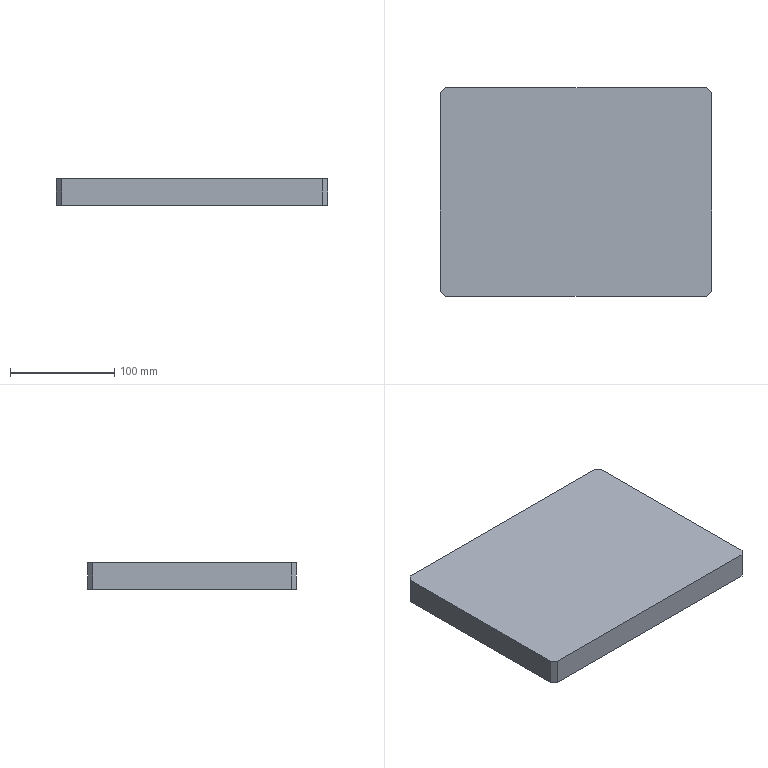Part | SolidWorks | features Chamfer 1, Extrusion 1 | 1 solid | 10 faces | box 260 x 200 x 25 mm | volume 1298750 mm3 | plane 10
STEP:
#1=CARTESIAN_POINT('',(130.,-95.,25.));
#2=VERTEX_POINT('',#1);
#3=CARTESIAN_POINT('',(130.,95.,25.));
#4=VERTEX_POINT('',#3);
#5=CARTESIAN_POINT('',(130.,100.,25.));
#6=DIRECTION('',(0.,1.,0.));
#7=VECTOR('',#6,1000.);
#8=LINE('',#5,#7);
#9=EDGE_CURVE('',#2,#4,#8,.T.);
#10=ORIENTED_EDGE('',*,*,#9,.F.);
#11=CARTESIAN_POINT('',(130.,-95.,0.));
#12=VERTEX_POINT('',#11);
#13=CARTESIAN_POINT('',(130.,-95.,25.));
#14=DIRECTION('',(0.,0.,-1.));
#15=VECTOR('',#14,1000.);
#16=LINE('',#13,#15);
#17=EDGE_CURVE('',#2,#12,#16,.T.);
#18=ORIENTED_EDGE('',*,*,#17,.T.);
#19=CARTESIAN_POINT('',(130.,95.,0.));
#20=VERTEX_POINT('',#19);
#21=CARTESIAN_POINT('',(130.,100.,0.));
#22=DIRECTION('',(0.,1.,0.));
#23=VECTOR('',#22,1000.);
#24=LINE('',#21,#23);
#25=EDGE_CURVE('',#12,#20,#24,.T.);
#26=ORIENTED_EDGE('',*,*,#25,.T.);
#27=CARTESIAN_POINT('',(130.,95.,25.));
#28=DIRECTION('',(0.,0.,1.));
#29=VECTOR('',#28,1000.);
#30=LINE('',#27,#29);
#31=EDGE_CURVE('',#20,#4,#30,.T.);
#32=ORIENTED_EDGE('',*,*,#31,.T.);
#33=EDGE_LOOP('',(#10,#18,#26,#32));
#34=FACE_OUTER_BOUND('',#33,.T.);
#35=CARTESIAN_POINT('',(130.,100.,25.));
#36=DIRECTION('',(-1.,0.,0.));
#37=DIRECTION('',(0.,-1.,0.));
#38=AXIS2_PLACEMENT_3D('',#35,#36,#37);
#39=PLANE('',#38);
#40=ADVANCED_FACE('',(#34),#39,.F.);
#41=CARTESIAN_POINT('',(125.,100.,0.));
#42=VERTEX_POINT('',#41);
#43=CARTESIAN_POINT('',(-125.,100.,0.));
#44=VERTEX_POINT('',#43);
#45=CARTESIAN_POINT('',(-130.,100.,0.));
#46=DIRECTION('',(-1.,0.,0.));
#47=VECTOR('',#46,1000.);
#48=LINE('',#45,#47);
#49=EDGE_CURVE('',#42,#44,#48,.T.);
#50=ORIENTED_EDGE('',*,*,#49,.T.);
#51=CARTESIAN_POINT('',(-125.,100.,25.));
#52=VERTEX_POINT('',#51);
#53=CARTESIAN_POINT('',(-125.,100.,25.));
#54=DIRECTION('',(0.,0.,1.));
#55=VECTOR('',#54,1000.);
#56=LINE('',#53,#55);
#57=EDGE_CURVE('',#44,#52,#56,.T.);
#58=ORIENTED_EDGE('',*,*,#57,.T.);
#59=CARTESIAN_POINT('',(125.,100.,25.));
#60=VERTEX_POINT('',#59);
#61=CARTESIAN_POINT('',(-130.,100.,25.));
#62=DIRECTION('',(-1.,0.,0.));
#63=VECTOR('',#62,1000.);
#64=LINE('',#61,#63);
#65=EDGE_CURVE('',#60,#52,#64,.T.);
#66=ORIENTED_EDGE('',*,*,#65,.F.);
#67=CARTESIAN_POINT('',(125.,100.,25.));
#68=DIRECTION('',(0.,0.,-1.));
#69=VECTOR('',#68,1000.);
#70=LINE('',#67,#69);
#71=EDGE_CURVE('',#60,#42,#70,.T.);
#72=ORIENTED_EDGE('',*,*,#71,.T.);
#73=EDGE_LOOP('',(#50,#58,#66,#72));
#74=FACE_OUTER_BOUND('',#73,.T.);
#75=CARTESIAN_POINT('',(-130.,100.,25.));
#76=DIRECTION('',(0.,-1.,0.));
#77=DIRECTION('',(0.,0.,-1.));
#78=AXIS2_PLACEMENT_3D('',#75,#76,#77);
#79=PLANE('',#78);
#80=ADVANCED_FACE('',(#74),#79,.F.);
#81=CARTESIAN_POINT('',(-130.,95.,0.));
#82=VERTEX_POINT('',#81);
#83=CARTESIAN_POINT('',(-130.,-95.,0.));
#84=VERTEX_POINT('',#83);
#85=CARTESIAN_POINT('',(-130.,100.,0.));
#86=DIRECTION('',(0.,-1.,0.));
#87=VECTOR('',#86,1000.);
#88=LINE('',#85,#87);
#89=EDGE_CURVE('',#82,#84,#88,.T.);
#90=ORIENTED_EDGE('',*,*,#89,.T.);
#91=CARTESIAN_POINT('',(-130.,-95.,25.));
#92=VERTEX_POINT('',#91);
#93=CARTESIAN_POINT('',(-130.,-95.,25.));
#94=DIRECTION('',(0.,0.,1.));
#95=VECTOR('',#94,1000.);
#96=LINE('',#93,#95);
#97=EDGE_CURVE('',#84,#92,#96,.T.);
#98=ORIENTED_EDGE('',*,*,#97,.T.);
#99=CARTESIAN_POINT('',(-130.,95.,25.));
#100=VERTEX_POINT('',#99);
#101=CARTESIAN_POINT('',(-130.,100.,25.));
#102=DIRECTION('',(0.,-1.,0.));
#103=VECTOR('',#102,1000.);
#104=LINE('',#101,#103);
#105=EDGE_CURVE('',#100,#92,#104,.T.);
#106=ORIENTED_EDGE('',*,*,#105,.F.);
#107=CARTESIAN_POINT('',(-130.,95.,25.));
#108=DIRECTION('',(0.,0.,-1.));
#109=VECTOR('',#108,1000.);
#110=LINE('',#107,#109);
#111=EDGE_CURVE('',#100,#82,#110,.T.);
#112=ORIENTED_EDGE('',*,*,#111,.T.);
#113=EDGE_LOOP('',(#90,#98,#106,#112));
#114=FACE_OUTER_BOUND('',#113,.T.);
#115=CARTESIAN_POINT('',(-130.,100.,25.));
#116=DIRECTION('',(1.,0.,0.));
#117=DIRECTION('',(0.,1.,0.));
#118=AXIS2_PLACEMENT_3D('',#115,#116,#117);
#119=PLANE('',#118);
#120=ADVANCED_FACE('',(#114),#119,.F.);
#121=CARTESIAN_POINT('',(-125.,-100.,25.));
#122=VERTEX_POINT('',#121);
#123=CARTESIAN_POINT('',(125.,-100.,25.));
#124=VERTEX_POINT('',#123);
#125=CARTESIAN_POINT('',(-130.,-100.,25.));
#126=DIRECTION('',(1.,0.,0.));
#127=VECTOR('',#126,1000.);
#128=LINE('',#125,#127);
#129=EDGE_CURVE('',#122,#124,#128,.T.);
#130=ORIENTED_EDGE('',*,*,#129,.F.);
#131=CARTESIAN_POINT('',(-125.,-100.,0.));
#132=VERTEX_POINT('',#131);
#133=CARTESIAN_POINT('',(-125.,-100.,25.));
#134=DIRECTION('',(0.,0.,-1.));
#135=VECTOR('',#134,1000.);
#136=LINE('',#133,#135);
#137=EDGE_CURVE('',#122,#132,#136,.T.);
#138=ORIENTED_EDGE('',*,*,#137,.T.);
#139=CARTESIAN_POINT('',(125.,-100.,0.));
#140=VERTEX_POINT('',#139);
#141=CARTESIAN_POINT('',(-130.,-100.,0.));
#142=DIRECTION('',(1.,0.,0.));
#143=VECTOR('',#142,1000.);
#144=LINE('',#141,#143);
#145=EDGE_CURVE('',#132,#140,#144,.T.);
#146=ORIENTED_EDGE('',*,*,#145,.T.);
#147=CARTESIAN_POINT('',(125.,-100.,25.));
#148=DIRECTION('',(0.,0.,1.));
#149=VECTOR('',#148,1000.);
#150=LINE('',#147,#149);
#151=EDGE_CURVE('',#140,#124,#150,.T.);
#152=ORIENTED_EDGE('',*,*,#151,.T.);
#153=EDGE_LOOP('',(#130,#138,#146,#152));
#154=FACE_OUTER_BOUND('',#153,.T.);
#155=CARTESIAN_POINT('',(-130.,-100.,25.));
#156=DIRECTION('',(0.,1.,0.));
#157=DIRECTION('',(0.,0.,1.));
#158=AXIS2_PLACEMENT_3D('',#155,#156,#157);
#159=PLANE('',#158);
#160=ADVANCED_FACE('',(#154),#159,.F.);
#161=ORIENTED_EDGE('',*,*,#105,.T.);
#162=CARTESIAN_POINT('',(-112.5,-112.5,25.));
#163=DIRECTION('',(0.7071,-0.7071,0.));
#164=VECTOR('',#163,1000.);
#165=LINE('',#162,#164);
#166=EDGE_CURVE('',#92,#122,#165,.T.);
#167=ORIENTED_EDGE('',*,*,#166,.T.);
#168=ORIENTED_EDGE('',*,*,#129,.T.);
#169=CARTESIAN_POINT('',(112.5,-112.5,25.));
#170=DIRECTION('',(0.7071,0.7071,0.));
#171=VECTOR('',#170,1000.);
#172=LINE('',#169,#171);
#173=EDGE_CURVE('',#124,#2,#172,.T.);
#174=ORIENTED_EDGE('',*,*,#173,.T.);
#175=ORIENTED_EDGE('',*,*,#9,.T.);
#176=CARTESIAN_POINT('',(112.5,112.5,25.));
#177=DIRECTION('',(-0.7071,0.7071,0.));
#178=VECTOR('',#177,1000.);
#179=LINE('',#176,#178);
#180=EDGE_CURVE('',#4,#60,#179,.T.);
#181=ORIENTED_EDGE('',*,*,#180,.T.);
#182=ORIENTED_EDGE('',*,*,#65,.T.);
#183=CARTESIAN_POINT('',(-112.5,112.5,25.));
#184=DIRECTION('',(-0.7071,-0.7071,0.));
#185=VECTOR('',#184,1000.);
#186=LINE('',#183,#185);
#187=EDGE_CURVE('',#52,#100,#186,.T.);
#188=ORIENTED_EDGE('',*,*,#187,.T.);
#189=EDGE_LOOP('',(#161,#167,#168,#174,#175,#181,#182,#188));
#190=FACE_OUTER_BOUND('',#189,.T.);
#191=CARTESIAN_POINT('',(0.,0.,25.));
#192=DIRECTION('',(0.,0.,1.));
#193=DIRECTION('',(1.,0.,0.));
#194=AXIS2_PLACEMENT_3D('',#191,#192,#193);
#195=PLANE('',#194);
#196=ADVANCED_FACE('',(#190),#195,.T.);
#197=ORIENTED_EDGE('',*,*,#145,.F.);
#198=CARTESIAN_POINT('',(-125.,-100.,0.));
#199=DIRECTION('',(-0.7071,0.7071,0.));
#200=VECTOR('',#199,1000.);
#201=LINE('',#198,#200);
#202=EDGE_CURVE('',#132,#84,#201,.T.);
#203=ORIENTED_EDGE('',*,*,#202,.T.);
#204=ORIENTED_EDGE('',*,*,#89,.F.);
#205=CARTESIAN_POINT('',(-130.,95.,0.));
#206=DIRECTION('',(0.7071,0.7071,0.));
#207=VECTOR('',#206,1000.);
#208=LINE('',#205,#207);
#209=EDGE_CURVE('',#82,#44,#208,.T.);
#210=ORIENTED_EDGE('',*,*,#209,.T.);
#211=ORIENTED_EDGE('',*,*,#49,.F.);
#212=CARTESIAN_POINT('',(125.,100.,0.));
#213=DIRECTION('',(0.7071,-0.7071,0.));
#214=VECTOR('',#213,1000.);
#215=LINE('',#212,#214);
#216=EDGE_CURVE('',#42,#20,#215,.T.);
#217=ORIENTED_EDGE('',*,*,#216,.T.);
#218=ORIENTED_EDGE('',*,*,#25,.F.);
#219=CARTESIAN_POINT('',(130.,-95.,0.));
#220=DIRECTION('',(-0.7071,-0.7071,0.));
#221=VECTOR('',#220,1000.);
#222=LINE('',#219,#221);
#223=EDGE_CURVE('',#12,#140,#222,.T.);
#224=ORIENTED_EDGE('',*,*,#223,.T.);
#225=EDGE_LOOP('',(#197,#203,#204,#210,#211,#217,#218,#224));
#226=FACE_OUTER_BOUND('',#225,.T.);
#227=CARTESIAN_POINT('',(0.,0.,0.));
#228=DIRECTION('',(0.,0.,1.));
#229=DIRECTION('',(1.,0.,0.));
#230=AXIS2_PLACEMENT_3D('',#227,#228,#229);
#231=PLANE('',#230);
#232=ADVANCED_FACE('',(#226),#231,.F.);
#233=ORIENTED_EDGE('',*,*,#166,.F.);
#234=ORIENTED_EDGE('',*,*,#97,.F.);
#235=ORIENTED_EDGE('',*,*,#202,.F.);
#236=ORIENTED_EDGE('',*,*,#137,.F.);
#237=EDGE_LOOP('',(#233,#234,#235,#236));
#238=FACE_OUTER_BOUND('',#237,.T.);
#239=CARTESIAN_POINT('',(-125.,-100.,25.));
#240=DIRECTION('',(0.7071,0.7071,0.));
#241=DIRECTION('',(0.,0.,-1.));
#242=AXIS2_PLACEMENT_3D('',#239,#240,#241);
#243=PLANE('',#242);
#244=ADVANCED_FACE('',(#238),#243,.F.);
#245=ORIENTED_EDGE('',*,*,#173,.F.);
#246=ORIENTED_EDGE('',*,*,#151,.F.);
#247=ORIENTED_EDGE('',*,*,#223,.F.);
#248=ORIENTED_EDGE('',*,*,#17,.F.);
#249=EDGE_LOOP('',(#245,#246,#247,#248));
#250=FACE_OUTER_BOUND('',#249,.T.);
#251=CARTESIAN_POINT('',(130.,-95.,25.));
#252=DIRECTION('',(-0.7071,0.7071,0.));
#253=DIRECTION('',(0.,0.,-1.));
#254=AXIS2_PLACEMENT_3D('',#251,#252,#253);
#255=PLANE('',#254);
#256=ADVANCED_FACE('',(#250),#255,.F.);
#257=ORIENTED_EDGE('',*,*,#187,.F.);
#258=ORIENTED_EDGE('',*,*,#57,.F.);
#259=ORIENTED_EDGE('',*,*,#209,.F.);
#260=ORIENTED_EDGE('',*,*,#111,.F.);
#261=EDGE_LOOP('',(#257,#258,#259,#260));
#262=FACE_OUTER_BOUND('',#261,.T.);
#263=CARTESIAN_POINT('',(-130.,95.,25.));
#264=DIRECTION('',(0.7071,-0.7071,0.));
#265=DIRECTION('',(0.,0.,-1.));
#266=AXIS2_PLACEMENT_3D('',#263,#264,#265);
#267=PLANE('',#266);
#268=ADVANCED_FACE('',(#262),#267,.F.);
#269=ORIENTED_EDGE('',*,*,#180,.F.);
#270=ORIENTED_EDGE('',*,*,#31,.F.);
#271=ORIENTED_EDGE('',*,*,#216,.F.);
#272=ORIENTED_EDGE('',*,*,#71,.F.);
#273=EDGE_LOOP('',(#269,#270,#271,#272));
#274=FACE_OUTER_BOUND('',#273,.T.);
#275=CARTESIAN_POINT('',(125.,100.,25.));
#276=DIRECTION('',(-0.7071,-0.7071,0.));
#277=DIRECTION('',(0.,0.,-1.));
#278=AXIS2_PLACEMENT_3D('',#275,#276,#277);
#279=PLANE('',#278);
#280=ADVANCED_FACE('',(#274),#279,.F.);
#281=CLOSED_SHELL('',(#40,#80,#120,#160,#196,#232,#244,#256,#268,#280));
#282=MANIFOLD_SOLID_BREP('',#281);
#283=CARTESIAN_POINT('',(0.,0.,0.));
#284=DIRECTION('',(0.,0.,1.));
#285=DIRECTION('',(1.,0.,0.));
#286=AXIS2_PLACEMENT_3D('',#283,#284,#285);
#287=(LENGTH_UNIT()NAMED_UNIT(*)SI_UNIT(.MILLI.,.METRE.));
#288=UNCERTAINTY_MEASURE_WITH_UNIT(LENGTH_MEASURE(0.00001),#287,'','');
#289=(NAMED_UNIT(*)PLANE_ANGLE_UNIT()SI_UNIT($,.RADIAN.));
#290=(NAMED_UNIT(*)SI_UNIT($,.STERADIAN.)SOLID_ANGLE_UNIT());
#291=(GEOMETRIC_REPRESENTATION_CONTEXT(3)GLOBAL_UNCERTAINTY_ASSIGNED_CONTEXT((#288))GLOBAL_UNIT_ASSIGNED_CONTEXT((#287,#289,#290))REPRESENTATION_CONTEXT('',''));
#292=ADVANCED_BREP_SHAPE_REPRESENTATION('',(#282,#286),#291);